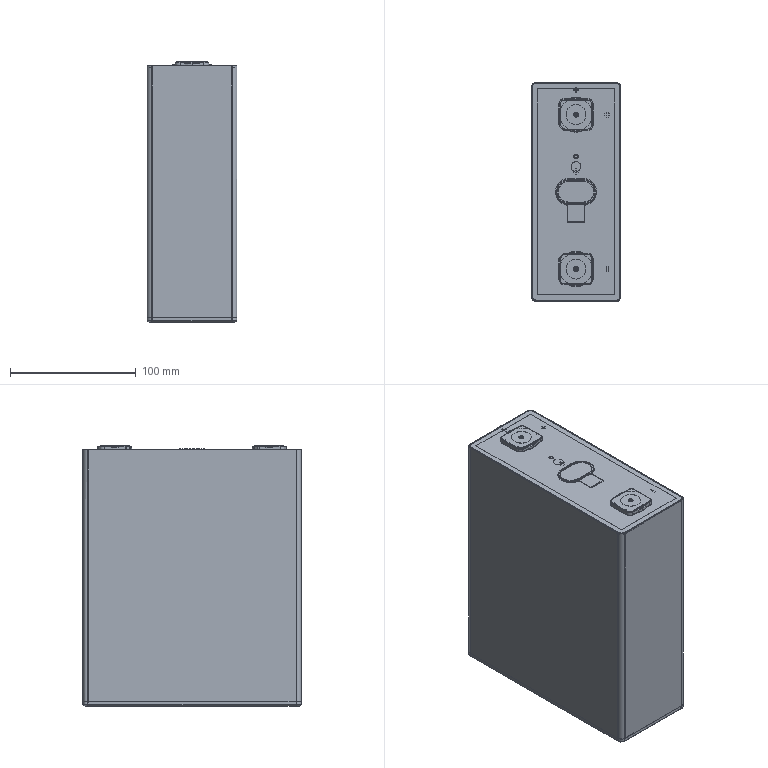Part | NX | features BREP 1 | 11 solids | 1053 faces | box 71.65 x 173.97 x 207.3 mm | volume 2687716 mm3 | plane 488 | cylinder 425 | torus 70 | cone 46 | spline 20 | sphere 4 | commonest cylinder face diameters 3 x72 6 x54 1 x42 2 x24 8 x18 4 x16